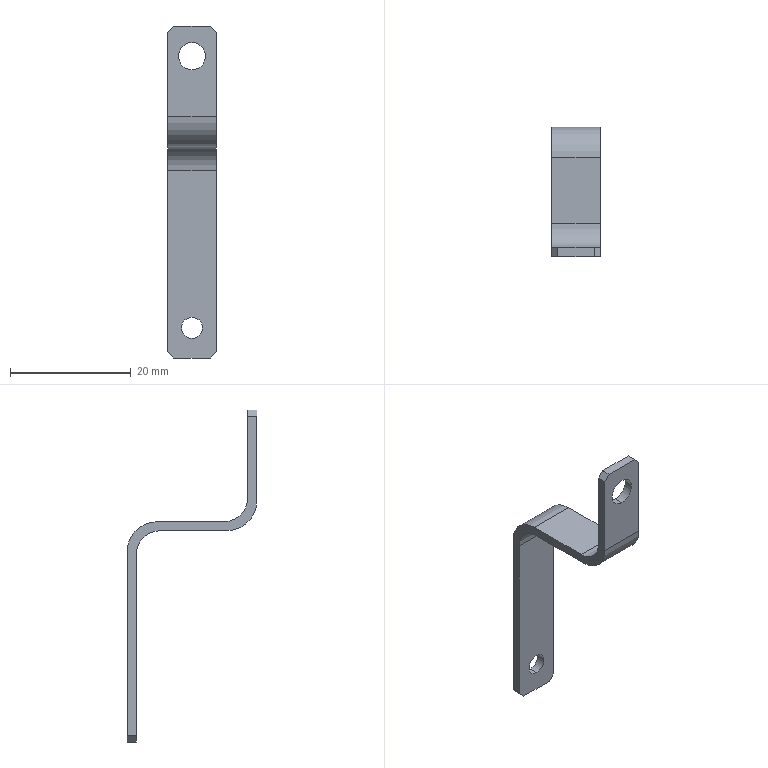Part | STEP file | 11-FG-B01411 | 1 solid | 22 faces | box 8 x 21.5 x 55 mm | volume 827.809 mm3 | plane 14 | cylinder 8 | commonest cylinder face diameters 3.5 x2 4.5 x2 8 x2 10 x2
STEP:
#1=CARTESIAN_POINT('',(4.,0.,-7.25));
#2=VERTEX_POINT('',#1);
#3=CARTESIAN_POINT('',(4.,0.,-2.75));
#4=VERTEX_POINT('',#3);
#5=CARTESIAN_POINT('',(4.,0.,-5.));
#6=DIRECTION('',(0.,1.,0.));
#7=DIRECTION('',(0.,0.,1.));
#8=AXIS2_PLACEMENT_3D('',#5,#6,#7);
#9=CIRCLE('',#8,2.25);
#10=EDGE_CURVE('',#2,#4,#9,.T.);
#11=ORIENTED_EDGE('',*,*,#10,.F.);
#12=CARTESIAN_POINT('',(4.,1.5,-7.25));
#13=VERTEX_POINT('',#12);
#14=CARTESIAN_POINT('',(4.,0.,-7.25));
#15=DIRECTION('',(0.,1.,0.));
#16=VECTOR('',#15,1000.);
#17=LINE('',#14,#16);
#18=EDGE_CURVE('',#2,#13,#17,.T.);
#19=ORIENTED_EDGE('',*,*,#18,.T.);
#20=CARTESIAN_POINT('',(4.,1.5,-2.75));
#21=VERTEX_POINT('',#20);
#22=CARTESIAN_POINT('',(4.,1.5,-5.));
#23=DIRECTION('',(0.,1.,0.));
#24=DIRECTION('',(0.,0.,1.));
#25=AXIS2_PLACEMENT_3D('',#22,#23,#24);
#26=CIRCLE('',#25,2.25);
#27=EDGE_CURVE('',#13,#21,#26,.T.);
#28=ORIENTED_EDGE('',*,*,#27,.T.);
#29=CARTESIAN_POINT('',(4.,0.,-2.75));
#30=DIRECTION('',(0.,1.,0.));
#31=VECTOR('',#30,1000.);
#32=LINE('',#29,#31);
#33=EDGE_CURVE('',#4,#21,#32,.T.);
#34=ORIENTED_EDGE('',*,*,#33,.F.);
#35=EDGE_LOOP('',(#11,#19,#28,#34));
#36=FACE_OUTER_BOUND('',#35,.T.);
#37=CARTESIAN_POINT('',(4.,0.,-5.));
#38=DIRECTION('',(0.,1.,0.));
#39=DIRECTION('',(0.,0.,1.));
#40=AXIS2_PLACEMENT_3D('',#37,#38,#39);
#41=CYLINDRICAL_SURFACE('',#40,2.25);
#42=ADVANCED_FACE('',(#36),#41,.F.);
#43=CARTESIAN_POINT('',(4.,20.,-51.75));
#44=VERTEX_POINT('',#43);
#45=CARTESIAN_POINT('',(4.,20.,-48.25));
#46=VERTEX_POINT('',#45);
#47=CARTESIAN_POINT('',(4.,20.,-50.));
#48=DIRECTION('',(0.,1.,0.));
#49=DIRECTION('',(0.,0.,1.));
#50=AXIS2_PLACEMENT_3D('',#47,#48,#49);
#51=CIRCLE('',#50,1.75);
#52=EDGE_CURVE('',#44,#46,#51,.T.);
#53=ORIENTED_EDGE('',*,*,#52,.F.);
#54=CARTESIAN_POINT('',(4.,21.5,-51.75));
#55=VERTEX_POINT('',#54);
#56=CARTESIAN_POINT('',(4.,0.,-51.75));
#57=DIRECTION('',(0.,1.,0.));
#58=VECTOR('',#57,1000.);
#59=LINE('',#56,#58);
#60=EDGE_CURVE('',#44,#55,#59,.T.);
#61=ORIENTED_EDGE('',*,*,#60,.T.);
#62=CARTESIAN_POINT('',(4.,21.5,-48.25));
#63=VERTEX_POINT('',#62);
#64=CARTESIAN_POINT('',(4.,21.5,-50.));
#65=DIRECTION('',(0.,1.,0.));
#66=DIRECTION('',(0.,0.,1.));
#67=AXIS2_PLACEMENT_3D('',#64,#65,#66);
#68=CIRCLE('',#67,1.75);
#69=EDGE_CURVE('',#55,#63,#68,.T.);
#70=ORIENTED_EDGE('',*,*,#69,.T.);
#71=CARTESIAN_POINT('',(4.,0.,-48.25));
#72=DIRECTION('',(0.,1.,0.));
#73=VECTOR('',#72,1000.);
#74=LINE('',#71,#73);
#75=EDGE_CURVE('',#46,#63,#74,.T.);
#76=ORIENTED_EDGE('',*,*,#75,.F.);
#77=EDGE_LOOP('',(#53,#61,#70,#76));
#78=FACE_OUTER_BOUND('',#77,.T.);
#79=CARTESIAN_POINT('',(4.,0.,-50.));
#80=DIRECTION('',(0.,1.,0.));
#81=DIRECTION('',(0.,0.,1.));
#82=AXIS2_PLACEMENT_3D('',#79,#80,#81);
#83=CYLINDRICAL_SURFACE('',#82,1.75);
#84=ADVANCED_FACE('',(#78),#83,.F.);
#85=CARTESIAN_POINT('',(8.,16.,-20.));
#86=VERTEX_POINT('',#85);
#87=CARTESIAN_POINT('',(8.,5.,-20.));
#88=VERTEX_POINT('',#87);
#89=CARTESIAN_POINT('',(8.,1.5,-20.));
#90=DIRECTION('',(0.,-1.,0.));
#91=VECTOR('',#90,1000.);
#92=LINE('',#89,#91);
#93=EDGE_CURVE('',#86,#88,#92,.T.);
#94=ORIENTED_EDGE('',*,*,#93,.T.);
#95=CARTESIAN_POINT('',(0.,5.,-20.));
#96=VERTEX_POINT('',#95);
#97=CARTESIAN_POINT('',(0.,5.,-20.));
#98=DIRECTION('',(-1.,0.,0.));
#99=VECTOR('',#98,1000.);
#100=LINE('',#97,#99);
#101=EDGE_CURVE('',#88,#96,#100,.T.);
#102=ORIENTED_EDGE('',*,*,#101,.T.);
#103=CARTESIAN_POINT('',(0.,16.,-20.));
#104=VERTEX_POINT('',#103);
#105=CARTESIAN_POINT('',(0.,1.5,-20.));
#106=DIRECTION('',(0.,-1.,0.));
#107=VECTOR('',#106,1000.);
#108=LINE('',#105,#107);
#109=EDGE_CURVE('',#104,#96,#108,.T.);
#110=ORIENTED_EDGE('',*,*,#109,.F.);
#111=CARTESIAN_POINT('',(8.,16.,-20.));
#112=DIRECTION('',(1.,0.,0.));
#113=VECTOR('',#112,1000.);
#114=LINE('',#111,#113);
#115=EDGE_CURVE('',#104,#86,#114,.T.);
#116=ORIENTED_EDGE('',*,*,#115,.T.);
#117=EDGE_LOOP('',(#94,#102,#110,#116));
#118=FACE_OUTER_BOUND('',#117,.T.);
#119=CARTESIAN_POINT('',(0.,1.5,-20.));
#120=DIRECTION('',(0.,0.,1.));
#121=DIRECTION('',(1.,0.,0.));
#122=AXIS2_PLACEMENT_3D('',#119,#120,#121);
#123=PLANE('',#122);
#124=ADVANCED_FACE('',(#118),#123,.F.);
#125=CARTESIAN_POINT('',(4.,1.5,-5.));
#126=DIRECTION('',(0.,1.,0.));
#127=DIRECTION('',(0.,0.,1.));
#128=AXIS2_PLACEMENT_3D('',#125,#126,#127);
#129=CIRCLE('',#128,2.25);
#130=EDGE_CURVE('',#21,#13,#129,.T.);
#131=ORIENTED_EDGE('',*,*,#130,.F.);
#132=ORIENTED_EDGE('',*,*,#27,.F.);
#133=EDGE_LOOP('',(#131,#132));
#134=FACE_BOUND('',#133,.T.);
#135=CARTESIAN_POINT('',(1.,1.5,0.));
#136=VERTEX_POINT('',#135);
#137=CARTESIAN_POINT('',(7.,1.5,0.));
#138=VERTEX_POINT('',#137);
#139=CARTESIAN_POINT('',(0.,1.5,0.));
#140=DIRECTION('',(1.,0.,0.));
#141=VECTOR('',#140,1000.);
#142=LINE('',#139,#141);
#143=EDGE_CURVE('',#136,#138,#142,.T.);
#144=ORIENTED_EDGE('',*,*,#143,.T.);
#145=CARTESIAN_POINT('',(8.,1.5,-1.));
#146=VERTEX_POINT('',#145);
#147=CARTESIAN_POINT('',(8.,1.5,-1.));
#148=DIRECTION('',(0.7071,0.,-0.7071));
#149=VECTOR('',#148,1000.);
#150=LINE('',#147,#149);
#151=EDGE_CURVE('',#138,#146,#150,.T.);
#152=ORIENTED_EDGE('',*,*,#151,.T.);
#153=CARTESIAN_POINT('',(8.,1.5,-14.5));
#154=VERTEX_POINT('',#153);
#155=CARTESIAN_POINT('',(8.,1.5,0.));
#156=DIRECTION('',(0.,0.,-1.));
#157=VECTOR('',#156,1000.);
#158=LINE('',#155,#157);
#159=EDGE_CURVE('',#146,#154,#158,.T.);
#160=ORIENTED_EDGE('',*,*,#159,.T.);
#161=CARTESIAN_POINT('',(0.,1.5,-14.5));
#162=VERTEX_POINT('',#161);
#163=CARTESIAN_POINT('',(0.,1.5,-14.5));
#164=DIRECTION('',(-1.,0.,0.));
#165=VECTOR('',#164,1000.);
#166=LINE('',#163,#165);
#167=EDGE_CURVE('',#154,#162,#166,.T.);
#168=ORIENTED_EDGE('',*,*,#167,.T.);
#169=CARTESIAN_POINT('',(0.,1.5,-1.));
#170=VERTEX_POINT('',#169);
#171=CARTESIAN_POINT('',(0.,1.5,0.));
#172=DIRECTION('',(0.,0.,1.));
#173=VECTOR('',#172,1000.);
#174=LINE('',#171,#173);
#175=EDGE_CURVE('',#162,#170,#174,.T.);
#176=ORIENTED_EDGE('',*,*,#175,.T.);
#177=CARTESIAN_POINT('',(1.,1.5,0.));
#178=DIRECTION('',(0.7071,0.,0.7071));
#179=VECTOR('',#178,1000.);
#180=LINE('',#177,#179);
#181=EDGE_CURVE('',#170,#136,#180,.T.);
#182=ORIENTED_EDGE('',*,*,#181,.T.);
#183=EDGE_LOOP('',(#144,#152,#160,#168,#176,#182));
#184=FACE_OUTER_BOUND('',#183,.T.);
#185=CARTESIAN_POINT('',(0.,1.5,0.));
#186=DIRECTION('',(0.,-1.,0.));
#187=DIRECTION('',(0.,0.,-1.));
#188=AXIS2_PLACEMENT_3D('',#185,#186,#187);
#189=PLANE('',#188);
#190=ADVANCED_FACE('',(#134,#184),#189,.F.);
#191=CARTESIAN_POINT('',(0.,0.,-15.));
#192=VERTEX_POINT('',#191);
#193=CARTESIAN_POINT('',(0.,0.,-1.));
#194=VERTEX_POINT('',#193);
#195=CARTESIAN_POINT('',(0.,0.,0.));
#196=DIRECTION('',(0.,0.,1.));
#197=VECTOR('',#196,1000.);
#198=LINE('',#195,#197);
#199=EDGE_CURVE('',#192,#194,#198,.T.);
#200=ORIENTED_EDGE('',*,*,#199,.T.);
#201=CARTESIAN_POINT('',(0.,1.5,-1.));
#202=DIRECTION('',(0.,1.,0.));
#203=VECTOR('',#202,1000.);
#204=LINE('',#201,#203);
#205=EDGE_CURVE('',#194,#170,#204,.T.);
#206=ORIENTED_EDGE('',*,*,#205,.T.);
#207=ORIENTED_EDGE('',*,*,#175,.F.);
#208=CARTESIAN_POINT('',(0.,5.5,-18.5));
#209=VERTEX_POINT('',#208);
#210=CARTESIAN_POINT('',(0.,5.5,-14.5));
#211=DIRECTION('',(1.,0.,0.));
#212=DIRECTION('',(0.,0.,-1.));
#213=AXIS2_PLACEMENT_3D('',#210,#211,#212);
#214=CIRCLE('',#213,4.);
#215=EDGE_CURVE('',#162,#209,#214,.T.);
#216=ORIENTED_EDGE('',*,*,#215,.T.);
#217=CARTESIAN_POINT('',(0.,16.5,-18.5));
#218=VERTEX_POINT('',#217);
#219=CARTESIAN_POINT('',(0.,21.5,-18.5));
#220=DIRECTION('',(0.,-1.,0.));
#221=VECTOR('',#220,1000.);
#222=LINE('',#219,#221);
#223=EDGE_CURVE('',#218,#209,#222,.T.);
#224=ORIENTED_EDGE('',*,*,#223,.F.);
#225=CARTESIAN_POINT('',(0.,21.5,-23.5));
#226=VERTEX_POINT('',#225);
#227=CARTESIAN_POINT('',(0.,16.5,-23.5));
#228=DIRECTION('',(-1.,0.,0.));
#229=DIRECTION('',(0.,0.,-1.));
#230=AXIS2_PLACEMENT_3D('',#227,#228,#229);
#231=CIRCLE('',#230,5.);
#232=EDGE_CURVE('',#218,#226,#231,.T.);
#233=ORIENTED_EDGE('',*,*,#232,.T.);
#234=CARTESIAN_POINT('',(0.,21.5,-54.));
#235=VERTEX_POINT('',#234);
#236=CARTESIAN_POINT('',(0.,21.5,-20.));
#237=DIRECTION('',(0.,0.,1.));
#238=VECTOR('',#237,1000.);
#239=LINE('',#236,#238);
#240=EDGE_CURVE('',#235,#226,#239,.T.);
#241=ORIENTED_EDGE('',*,*,#240,.F.);
#242=CARTESIAN_POINT('',(0.,20.,-54.));
#243=VERTEX_POINT('',#242);
#244=CARTESIAN_POINT('',(0.,20.,-54.));
#245=DIRECTION('',(0.,-1.,0.));
#246=VECTOR('',#245,1000.);
#247=LINE('',#244,#246);
#248=EDGE_CURVE('',#235,#243,#247,.T.);
#249=ORIENTED_EDGE('',*,*,#248,.T.);
#250=CARTESIAN_POINT('',(0.,20.,-24.));
#251=VERTEX_POINT('',#250);
#252=CARTESIAN_POINT('',(0.,20.,-55.));
#253=DIRECTION('',(0.,0.,1.));
#254=VECTOR('',#253,1000.);
#255=LINE('',#252,#254);
#256=EDGE_CURVE('',#243,#251,#255,.T.);
#257=ORIENTED_EDGE('',*,*,#256,.T.);
#258=CARTESIAN_POINT('',(0.,16.,-24.));
#259=DIRECTION('',(1.,0.,0.));
#260=DIRECTION('',(0.,0.,-1.));
#261=AXIS2_PLACEMENT_3D('',#258,#259,#260);
#262=CIRCLE('',#261,4.);
#263=EDGE_CURVE('',#251,#104,#262,.T.);
#264=ORIENTED_EDGE('',*,*,#263,.T.);
#265=ORIENTED_EDGE('',*,*,#109,.T.);
#266=CARTESIAN_POINT('',(0.,5.,-15.));
#267=DIRECTION('',(-1.,0.,0.));
#268=DIRECTION('',(0.,0.,-1.));
#269=AXIS2_PLACEMENT_3D('',#266,#267,#268);
#270=CIRCLE('',#269,5.);
#271=EDGE_CURVE('',#96,#192,#270,.T.);
#272=ORIENTED_EDGE('',*,*,#271,.T.);
#273=EDGE_LOOP('',(#200,#206,#207,#216,#224,#233,#241,#249,#257,#264,#265,#272));
#274=FACE_OUTER_BOUND('',#273,.T.);
#275=CARTESIAN_POINT('',(0.,1.5,0.));
#276=DIRECTION('',(1.,0.,0.));
#277=DIRECTION('',(0.,0.,-1.));
#278=AXIS2_PLACEMENT_3D('',#275,#276,#277);
#279=PLANE('',#278);
#280=ADVANCED_FACE('',(#274),#279,.F.);
#281=CARTESIAN_POINT('',(1.,0.,0.));
#282=VERTEX_POINT('',#281);
#283=CARTESIAN_POINT('',(7.,0.,0.));
#284=VERTEX_POINT('',#283);
#285=CARTESIAN_POINT('',(0.,0.,0.));
#286=DIRECTION('',(1.,0.,0.));
#287=VECTOR('',#286,1000.);
#288=LINE('',#285,#287);
#289=EDGE_CURVE('',#282,#284,#288,.T.);
#290=ORIENTED_EDGE('',*,*,#289,.T.);
#291=CARTESIAN_POINT('',(7.,1.5,0.));
#292=DIRECTION('',(0.,1.,0.));
#293=VECTOR('',#292,1000.);
#294=LINE('',#291,#293);
#295=EDGE_CURVE('',#284,#138,#294,.T.);
#296=ORIENTED_EDGE('',*,*,#295,.T.);
#297=ORIENTED_EDGE('',*,*,#143,.F.);
#298=CARTESIAN_POINT('',(1.,1.5,0.));
#299=DIRECTION('',(0.,-1.,0.));
#300=VECTOR('',#299,1000.);
#301=LINE('',#298,#300);
#302=EDGE_CURVE('',#136,#282,#301,.T.);
#303=ORIENTED_EDGE('',*,*,#302,.T.);
#304=EDGE_LOOP('',(#290,#296,#297,#303));
#305=FACE_OUTER_BOUND('',#304,.T.);
#306=CARTESIAN_POINT('',(0.,1.5,0.));
#307=DIRECTION('',(0.,0.,-1.));
#308=DIRECTION('',(-1.,0.,0.));
#309=AXIS2_PLACEMENT_3D('',#306,#307,#308);
#310=PLANE('',#309);
#311=ADVANCED_FACE('',(#305),#310,.F.);
#312=ORIENTED_EDGE('',*,*,#159,.F.);
#313=CARTESIAN_POINT('',(8.,0.,-1.));
#314=VERTEX_POINT('',#313);
#315=CARTESIAN_POINT('',(8.,1.5,-1.));
#316=DIRECTION('',(0.,-1.,0.));
#317=VECTOR('',#316,1000.);
#318=LINE('',#315,#317);
#319=EDGE_CURVE('',#146,#314,#318,.T.);
#320=ORIENTED_EDGE('',*,*,#319,.T.);
#321=CARTESIAN_POINT('',(8.,0.,-15.));
#322=VERTEX_POINT('',#321);
#323=CARTESIAN_POINT('',(8.,0.,0.));
#324=DIRECTION('',(0.,0.,-1.));
#325=VECTOR('',#324,1000.);
#326=LINE('',#323,#325);
#327=EDGE_CURVE('',#314,#322,#326,.T.);
#328=ORIENTED_EDGE('',*,*,#327,.T.);
#329=CARTESIAN_POINT('',(8.,5.,-15.));
#330=DIRECTION('',(1.,0.,0.));
#331=DIRECTION('',(0.,0.,1.));
#332=AXIS2_PLACEMENT_3D('',#329,#330,#331);
#333=CIRCLE('',#332,5.);
#334=EDGE_CURVE('',#322,#88,#333,.T.);
#335=ORIENTED_EDGE('',*,*,#334,.T.);
#336=ORIENTED_EDGE('',*,*,#93,.F.);
#337=CARTESIAN_POINT('',(8.,20.,-24.));
#338=VERTEX_POINT('',#337);
#339=CARTESIAN_POINT('',(8.,16.,-24.));
#340=DIRECTION('',(-1.,0.,0.));
#341=DIRECTION('',(0.,0.,1.));
#342=AXIS2_PLACEMENT_3D('',#339,#340,#341);
#343=CIRCLE('',#342,4.);
#344=EDGE_CURVE('',#86,#338,#343,.T.);
#345=ORIENTED_EDGE('',*,*,#344,.T.);
#346=CARTESIAN_POINT('',(8.,20.,-54.));
#347=VERTEX_POINT('',#346);
#348=CARTESIAN_POINT('',(8.,20.,-55.));
#349=DIRECTION('',(0.,0.,1.));
#350=VECTOR('',#349,1000.);
#351=LINE('',#348,#350);
#352=EDGE_CURVE('',#347,#338,#351,.T.);
#353=ORIENTED_EDGE('',*,*,#352,.F.);
#354=CARTESIAN_POINT('',(8.,21.5,-54.));
#355=VERTEX_POINT('',#354);
#356=CARTESIAN_POINT('',(8.,21.5,-54.));
#357=DIRECTION('',(0.,1.,0.));
#358=VECTOR('',#357,1000.);
#359=LINE('',#356,#358);
#360=EDGE_CURVE('',#347,#355,#359,.T.);
#361=ORIENTED_EDGE('',*,*,#360,.T.);
#362=CARTESIAN_POINT('',(8.,21.5,-23.5));
#363=VERTEX_POINT('',#362);
#364=CARTESIAN_POINT('',(8.,21.5,-20.));
#365=DIRECTION('',(0.,0.,-1.));
#366=VECTOR('',#365,1000.);
#367=LINE('',#364,#366);
#368=EDGE_CURVE('',#363,#355,#367,.T.);
#369=ORIENTED_EDGE('',*,*,#368,.F.);
#370=CARTESIAN_POINT('',(8.,16.5,-18.5));
#371=VERTEX_POINT('',#370);
#372=CARTESIAN_POINT('',(8.,16.5,-23.5));
#373=DIRECTION('',(1.,0.,0.));
#374=DIRECTION('',(0.,0.,1.));
#375=AXIS2_PLACEMENT_3D('',#372,#373,#374);
#376=CIRCLE('',#375,5.);
#377=EDGE_CURVE('',#363,#371,#376,.T.);
#378=ORIENTED_EDGE('',*,*,#377,.T.);
#379=CARTESIAN_POINT('',(8.,5.5,-18.5));
#380=VERTEX_POINT('',#379);
#381=CARTESIAN_POINT('',(8.,21.5,-18.5));
#382=DIRECTION('',(0.,-1.,0.));
#383=VECTOR('',#382,1000.);
#384=LINE('',#381,#383);
#385=EDGE_CURVE('',#371,#380,#384,.T.);
#386=ORIENTED_EDGE('',*,*,#385,.T.);
#387=CARTESIAN_POINT('',(8.,5.5,-14.5));
#388=DIRECTION('',(-1.,0.,0.));
#389=DIRECTION('',(0.,0.,1.));
#390=AXIS2_PLACEMENT_3D('',#387,#388,#389);
#391=CIRCLE('',#390,4.);
#392=EDGE_CURVE('',#380,#154,#391,.T.);
#393=ORIENTED_EDGE('',*,*,#392,.T.);
#394=EDGE_LOOP('',(#312,#320,#328,#335,#336,#345,#353,#361,#369,#378,#386,#393));
#395=FACE_OUTER_BOUND('',#394,.T.);
#396=CARTESIAN_POINT('',(8.,1.5,0.));
#397=DIRECTION('',(-1.,0.,0.));
#398=DIRECTION('',(0.,0.,1.));
#399=AXIS2_PLACEMENT_3D('',#396,#397,#398);
#400=PLANE('',#399);
#401=ADVANCED_FACE('',(#395),#400,.F.);
#402=CARTESIAN_POINT('',(4.,0.,-5.));
#403=DIRECTION('',(0.,1.,0.));
#404=DIRECTION('',(0.,0.,1.));
#405=AXIS2_PLACEMENT_3D('',#402,#403,#404);
#406=CIRCLE('',#405,2.25);
#407=EDGE_CURVE('',#4,#2,#406,.T.);
#408=ORIENTED_EDGE('',*,*,#407,.T.);
#409=ORIENTED_EDGE('',*,*,#10,.T.);
#410=EDGE_LOOP('',(#408,#409));
#411=FACE_BOUND('',#410,.T.);
#412=ORIENTED_EDGE('',*,*,#327,.F.);
#413=CARTESIAN_POINT('',(3.5,0.,3.5));
#414=DIRECTION('',(-0.7071,0.,0.7071));
#415=VECTOR('',#414,1000.);
#416=LINE('',#413,#415);
#417=EDGE_CURVE('',#314,#284,#416,.T.);
#418=ORIENTED_EDGE('',*,*,#417,.T.);
#419=ORIENTED_EDGE('',*,*,#289,.F.);
#420=CARTESIAN_POINT('',(0.5,0.,-0.5));
#421=DIRECTION('',(-0.7071,0.,-0.7071));
#422=VECTOR('',#421,1000.);
#423=LINE('',#420,#422);
#424=EDGE_CURVE('',#282,#194,#423,.T.);
#425=ORIENTED_EDGE('',*,*,#424,.T.);
#426=ORIENTED_EDGE('',*,*,#199,.F.);
#427=CARTESIAN_POINT('',(8.,0.,-15.));
#428=DIRECTION('',(1.,0.,0.));
#429=VECTOR('',#428,1000.);
#430=LINE('',#427,#429);
#431=EDGE_CURVE('',#192,#322,#430,.T.);
#432=ORIENTED_EDGE('',*,*,#431,.T.);
#433=EDGE_LOOP('',(#412,#418,#419,#425,#426,#432));
#434=FACE_OUTER_BOUND('',#433,.T.);
#435=CARTESIAN_POINT('',(0.,0.,0.));
#436=DIRECTION('',(0.,-1.,0.));
#437=DIRECTION('',(0.,0.,-1.));
#438=AXIS2_PLACEMENT_3D('',#435,#436,#437);
#439=PLANE('',#438);
#440=ADVANCED_FACE('',(#411,#434),#439,.T.);
#441=ORIENTED_EDGE('',*,*,#385,.F.);
#442=CARTESIAN_POINT('',(0.,16.5,-18.5));
#443=DIRECTION('',(-1.,0.,0.));
#444=VECTOR('',#443,1000.);
#445=LINE('',#442,#444);
#446=EDGE_CURVE('',#371,#218,#445,.T.);
#447=ORIENTED_EDGE('',*,*,#446,.T.);
#448=ORIENTED_EDGE('',*,*,#223,.T.);
#449=CARTESIAN_POINT('',(8.,5.5,-18.5));
#450=DIRECTION('',(1.,0.,0.));
#451=VECTOR('',#450,1000.);
#452=LINE('',#449,#451);
#453=EDGE_CURVE('',#209,#380,#452,.T.);
#454=ORIENTED_EDGE('',*,*,#453,.T.);
#455=EDGE_LOOP('',(#441,#447,#448,#454));
#456=FACE_OUTER_BOUND('',#455,.T.);
#457=CARTESIAN_POINT('',(0.,21.5,-18.5));
#458=DIRECTION('',(0.,0.,-1.));
#459=DIRECTION('',(-1.,0.,0.));
#460=AXIS2_PLACEMENT_3D('',#457,#458,#459);
#461=PLANE('',#460);
#462=ADVANCED_FACE('',(#456),#461,.F.);
#463=CARTESIAN_POINT('',(4.,21.5,-50.));
#464=DIRECTION('',(0.,1.,0.));
#465=DIRECTION('',(0.,0.,1.));
#466=AXIS2_PLACEMENT_3D('',#463,#464,#465);
#467=CIRCLE('',#466,1.75);
#468=EDGE_CURVE('',#63,#55,#467,.T.);
#469=ORIENTED_EDGE('',*,*,#468,.F.);
#470=ORIENTED_EDGE('',*,*,#69,.F.);
#471=EDGE_LOOP('',(#469,#470));
#472=FACE_BOUND('',#471,.T.);
#473=CARTESIAN_POINT('',(1.,21.5,-55.));
#474=VERTEX_POINT('',#473);
#475=CARTESIAN_POINT('',(7.,21.5,-55.));
#476=VERTEX_POINT('',#475);
#477=CARTESIAN_POINT('',(8.,21.5,-55.));
#478=DIRECTION('',(1.,0.,0.));
#479=VECTOR('',#478,1000.);
#480=LINE('',#477,#479);
#481=EDGE_CURVE('',#474,#476,#480,.T.);
#482=ORIENTED_EDGE('',*,*,#481,.F.);
#483=CARTESIAN_POINT('',(-27.,21.5,-27.));
#484=DIRECTION('',(-0.7071,0.,0.7071));
#485=VECTOR('',#484,1000.);
#486=LINE('',#483,#485);
#487=EDGE_CURVE('',#474,#235,#486,.T.);
#488=ORIENTED_EDGE('',*,*,#487,.T.);
#489=ORIENTED_EDGE('',*,*,#240,.T.);
#490=CARTESIAN_POINT('',(8.,21.5,-23.5));
#491=DIRECTION('',(1.,0.,0.));
#492=VECTOR('',#491,1000.);
#493=LINE('',#490,#492);
#494=EDGE_CURVE('',#226,#363,#493,.T.);
#495=ORIENTED_EDGE('',*,*,#494,.T.);
#496=ORIENTED_EDGE('',*,*,#368,.T.);
#497=CARTESIAN_POINT('',(31.,21.5,-31.));
#498=DIRECTION('',(-0.7071,0.,-0.7071));
#499=VECTOR('',#498,1000.);
#500=LINE('',#497,#499);
#501=EDGE_CURVE('',#355,#476,#500,.T.);
#502=ORIENTED_EDGE('',*,*,#501,.T.);
#503=EDGE_LOOP('',(#482,#488,#489,#495,#496,#502));
#504=FACE_OUTER_BOUND('',#503,.T.);
#505=CARTESIAN_POINT('',(0.,21.5,0.));
#506=DIRECTION('',(0.,1.,0.));
#507=DIRECTION('',(0.,0.,1.));
#508=AXIS2_PLACEMENT_3D('',#505,#506,#507);
#509=PLANE('',#508);
#510=ADVANCED_FACE('',(#472,#504),#509,.T.);
#511=CARTESIAN_POINT('',(4.,20.,-50.));
#512=DIRECTION('',(0.,1.,0.));
#513=DIRECTION('',(0.,0.,1.));
#514=AXIS2_PLACEMENT_3D('',#511,#512,#513);
#515=CIRCLE('',#514,1.75);
#516=EDGE_CURVE('',#46,#44,#515,.T.);
#517=ORIENTED_EDGE('',*,*,#516,.T.);
#518=ORIENTED_EDGE('',*,*,#52,.T.);
#519=EDGE_LOOP('',(#517,#518));
#520=FACE_BOUND('',#519,.T.);
#521=ORIENTED_EDGE('',*,*,#256,.F.);
#522=CARTESIAN_POINT('',(1.,20.,-55.));
#523=VERTEX_POINT('',#522);
#524=CARTESIAN_POINT('',(1.,20.,-55.));
#525=DIRECTION('',(0.7071,0.,-0.7071));
#526=VECTOR('',#525,1000.);
#527=LINE('',#524,#526);
#528=EDGE_CURVE('',#243,#523,#527,.T.);
#529=ORIENTED_EDGE('',*,*,#528,.T.);
#530=CARTESIAN_POINT('',(7.,20.,-55.));
#531=VERTEX_POINT('',#530);
#532=CARTESIAN_POINT('',(8.,20.,-55.));
#533=DIRECTION('',(-1.,0.,0.));
#534=VECTOR('',#533,1000.);
#535=LINE('',#532,#534);
#536=EDGE_CURVE('',#531,#523,#535,.T.);
#537=ORIENTED_EDGE('',*,*,#536,.F.);
#538=CARTESIAN_POINT('',(7.,20.,-55.));
#539=DIRECTION('',(0.7071,0.,0.7071));
#540=VECTOR('',#539,1000.);
#541=LINE('',#538,#540);
#542=EDGE_CURVE('',#531,#347,#541,.T.);
#543=ORIENTED_EDGE('',*,*,#542,.T.);
#544=ORIENTED_EDGE('',*,*,#352,.T.);
#545=CARTESIAN_POINT('',(0.,20.,-24.));
#546=DIRECTION('',(-1.,0.,0.));
#547=VECTOR('',#546,1000.);
#548=LINE('',#545,#547);
#549=EDGE_CURVE('',#338,#251,#548,.T.);
#550=ORIENTED_EDGE('',*,*,#549,.T.);
#551=EDGE_LOOP('',(#521,#529,#537,#543,#544,#550));
#552=FACE_OUTER_BOUND('',#551,.T.);
#553=CARTESIAN_POINT('',(8.,20.,-55.));
#554=DIRECTION('',(0.,1.,0.));
#555=DIRECTION('',(0.,0.,1.));
#556=AXIS2_PLACEMENT_3D('',#553,#554,#555);
#557=PLANE('',#556);
#558=ADVANCED_FACE('',(#520,#552),#557,.F.);
#559=ORIENTED_EDGE('',*,*,#536,.T.);
#560=CARTESIAN_POINT('',(1.,21.5,-55.));
#561=DIRECTION('',(0.,1.,0.));
#562=VECTOR('',#561,1000.);
#563=LINE('',#560,#562);
#564=EDGE_CURVE('',#523,#474,#563,.T.);
#565=ORIENTED_EDGE('',*,*,#564,.T.);
#566=ORIENTED_EDGE('',*,*,#481,.T.);
#567=CARTESIAN_POINT('',(7.,20.,-55.));
#568=DIRECTION('',(0.,-1.,0.));
#569=VECTOR('',#568,1000.);
#570=LINE('',#567,#569);
#571=EDGE_CURVE('',#476,#531,#570,.T.);
#572=ORIENTED_EDGE('',*,*,#571,.T.);
#573=EDGE_LOOP('',(#559,#565,#566,#572));
#574=FACE_OUTER_BOUND('',#573,.T.);
#575=CARTESIAN_POINT('',(0.,0.,-55.));
#576=DIRECTION('',(0.,0.,-1.));
#577=DIRECTION('',(-1.,0.,0.));
#578=AXIS2_PLACEMENT_3D('',#575,#576,#577);
#579=PLANE('',#578);
#580=ADVANCED_FACE('',(#574),#579,.T.);
#581=ORIENTED_EDGE('',*,*,#344,.F.);
#582=ORIENTED_EDGE('',*,*,#115,.F.);
#583=ORIENTED_EDGE('',*,*,#263,.F.);
#584=ORIENTED_EDGE('',*,*,#549,.F.);
#585=EDGE_LOOP('',(#581,#582,#583,#584));
#586=FACE_OUTER_BOUND('',#585,.T.);
#587=CARTESIAN_POINT('',(8.,16.,-24.));
#588=DIRECTION('',(1.,0.,0.));
#589=DIRECTION('',(0.,0.,-1.));
#590=AXIS2_PLACEMENT_3D('',#587,#588,#589);
#591=CYLINDRICAL_SURFACE('',#590,4.);
#592=ADVANCED_FACE('',(#586),#591,.F.);
#593=ORIENTED_EDGE('',*,*,#215,.F.);
#594=ORIENTED_EDGE('',*,*,#167,.F.);
#595=ORIENTED_EDGE('',*,*,#392,.F.);
#596=ORIENTED_EDGE('',*,*,#453,.F.);
#597=EDGE_LOOP('',(#593,#594,#595,#596));
#598=FACE_OUTER_BOUND('',#597,.T.);
#599=CARTESIAN_POINT('',(0.,5.5,-14.5));
#600=DIRECTION('',(-1.,0.,0.));
#601=DIRECTION('',(0.,0.,1.));
#602=AXIS2_PLACEMENT_3D('',#599,#600,#601);
#603=CYLINDRICAL_SURFACE('',#602,4.);
#604=ADVANCED_FACE('',(#598),#603,.F.);
#605=ORIENTED_EDGE('',*,*,#334,.F.);
#606=ORIENTED_EDGE('',*,*,#431,.F.);
#607=ORIENTED_EDGE('',*,*,#271,.F.);
#608=ORIENTED_EDGE('',*,*,#101,.F.);
#609=EDGE_LOOP('',(#605,#606,#607,#608));
#610=FACE_OUTER_BOUND('',#609,.T.);
#611=CARTESIAN_POINT('',(0.,5.,-15.));
#612=DIRECTION('',(1.,0.,0.));
#613=DIRECTION('',(0.,0.,-1.));
#614=AXIS2_PLACEMENT_3D('',#611,#612,#613);
#615=CYLINDRICAL_SURFACE('',#614,5.);
#616=ADVANCED_FACE('',(#610),#615,.T.);
#617=ORIENTED_EDGE('',*,*,#232,.F.);
#618=ORIENTED_EDGE('',*,*,#446,.F.);
#619=ORIENTED_EDGE('',*,*,#377,.F.);
#620=ORIENTED_EDGE('',*,*,#494,.F.);
#621=EDGE_LOOP('',(#617,#618,#619,#620));
#622=FACE_OUTER_BOUND('',#621,.T.);
#623=CARTESIAN_POINT('',(0.,16.5,-23.5));
#624=DIRECTION('',(-1.,0.,0.));
#625=DIRECTION('',(0.,0.,1.));
#626=AXIS2_PLACEMENT_3D('',#623,#624,#625);
#627=CYLINDRICAL_SURFACE('',#626,5.);
#628=ADVANCED_FACE('',(#622),#627,.T.);
#629=ORIENTED_EDGE('',*,*,#60,.F.);
#630=ORIENTED_EDGE('',*,*,#516,.F.);
#631=ORIENTED_EDGE('',*,*,#75,.T.);
#632=ORIENTED_EDGE('',*,*,#468,.T.);
#633=EDGE_LOOP('',(#629,#630,#631,#632));
#634=FACE_OUTER_BOUND('',#633,.T.);
#635=CARTESIAN_POINT('',(4.,0.,-50.));
#636=DIRECTION('',(0.,1.,0.));
#637=DIRECTION('',(0.,0.,1.));
#638=AXIS2_PLACEMENT_3D('',#635,#636,#637);
#639=CYLINDRICAL_SURFACE('',#638,1.75);
#640=ADVANCED_FACE('',(#634),#639,.F.);
#641=ORIENTED_EDGE('',*,*,#528,.F.);
#642=ORIENTED_EDGE('',*,*,#248,.F.);
#643=ORIENTED_EDGE('',*,*,#487,.F.);
#644=ORIENTED_EDGE('',*,*,#564,.F.);
#645=EDGE_LOOP('',(#641,#642,#643,#644));
#646=FACE_OUTER_BOUND('',#645,.T.);
#647=CARTESIAN_POINT('',(1.,0.,-55.));
#648=DIRECTION('',(-0.7071,0.,-0.7071));
#649=DIRECTION('',(0.,-1.,0.));
#650=AXIS2_PLACEMENT_3D('',#647,#648,#649);
#651=PLANE('',#650);
#652=ADVANCED_FACE('',(#646),#651,.T.);
#653=ORIENTED_EDGE('',*,*,#501,.F.);
#654=ORIENTED_EDGE('',*,*,#360,.F.);
#655=ORIENTED_EDGE('',*,*,#542,.F.);
#656=ORIENTED_EDGE('',*,*,#571,.F.);
#657=EDGE_LOOP('',(#653,#654,#655,#656));
#658=FACE_OUTER_BOUND('',#657,.T.);
#659=CARTESIAN_POINT('',(7.,0.,-55.));
#660=DIRECTION('',(0.7071,0.,-0.7071));
#661=DIRECTION('',(0.,1.,0.));
#662=AXIS2_PLACEMENT_3D('',#659,#660,#661);
#663=PLANE('',#662);
#664=ADVANCED_FACE('',(#658),#663,.T.);
#665=ORIENTED_EDGE('',*,*,#18,.F.);
#666=ORIENTED_EDGE('',*,*,#407,.F.);
#667=ORIENTED_EDGE('',*,*,#33,.T.);
#668=ORIENTED_EDGE('',*,*,#130,.T.);
#669=EDGE_LOOP('',(#665,#666,#667,#668));
#670=FACE_OUTER_BOUND('',#669,.T.);
#671=CARTESIAN_POINT('',(4.,0.,-5.));
#672=DIRECTION('',(0.,1.,0.));
#673=DIRECTION('',(0.,0.,1.));
#674=AXIS2_PLACEMENT_3D('',#671,#672,#673);
#675=CYLINDRICAL_SURFACE('',#674,2.25);
#676=ADVANCED_FACE('',(#670),#675,.F.);
#677=ORIENTED_EDGE('',*,*,#151,.F.);
#678=ORIENTED_EDGE('',*,*,#295,.F.);
#679=ORIENTED_EDGE('',*,*,#417,.F.);
#680=ORIENTED_EDGE('',*,*,#319,.F.);
#681=EDGE_LOOP('',(#677,#678,#679,#680));
#682=FACE_OUTER_BOUND('',#681,.T.);
#683=CARTESIAN_POINT('',(8.,1.5,-1.));
#684=DIRECTION('',(-0.7071,0.,-0.7071));
#685=DIRECTION('',(0.,-1.,0.));
#686=AXIS2_PLACEMENT_3D('',#683,#684,#685);
#687=PLANE('',#686);
#688=ADVANCED_FACE('',(#682),#687,.F.);
#689=ORIENTED_EDGE('',*,*,#181,.F.);
#690=ORIENTED_EDGE('',*,*,#205,.F.);
#691=ORIENTED_EDGE('',*,*,#424,.F.);
#692=ORIENTED_EDGE('',*,*,#302,.F.);
#693=EDGE_LOOP('',(#689,#690,#691,#692));
#694=FACE_OUTER_BOUND('',#693,.T.);
#695=CARTESIAN_POINT('',(1.,1.5,0.));
#696=DIRECTION('',(0.7071,0.,-0.7071));
#697=DIRECTION('',(0.,-1.,0.));
#698=AXIS2_PLACEMENT_3D('',#695,#696,#697);
#699=PLANE('',#698);
#700=ADVANCED_FACE('',(#694),#699,.F.);
#701=CLOSED_SHELL('',(#42,#84,#124,#190,#280,#311,#401,#440,#462,#510,#558,#580,#592,#604,#616,#628,#640,#652,#664,#676,#688,#700));
#702=MANIFOLD_SOLID_BREP('',#701);
#703=CARTESIAN_POINT('',(0.,0.,0.));
#704=DIRECTION('',(0.,0.,1.));
#705=DIRECTION('',(1.,0.,0.));
#706=AXIS2_PLACEMENT_3D('',#703,#704,#705);
#707=(LENGTH_UNIT()NAMED_UNIT(*)SI_UNIT(.MILLI.,.METRE.));
#708=UNCERTAINTY_MEASURE_WITH_UNIT(LENGTH_MEASURE(0.00001),#707,'','');
#709=(NAMED_UNIT(*)PLANE_ANGLE_UNIT()SI_UNIT($,.RADIAN.));
#710=(NAMED_UNIT(*)SI_UNIT($,.STERADIAN.)SOLID_ANGLE_UNIT());
#711=(GEOMETRIC_REPRESENTATION_CONTEXT(3)GLOBAL_UNCERTAINTY_ASSIGNED_CONTEXT((#708))GLOBAL_UNIT_ASSIGNED_CONTEXT((#707,#709,#710))REPRESENTATION_CONTEXT('',''));
#712=ADVANCED_BREP_SHAPE_REPRESENTATION('',(#702,#706),#711);